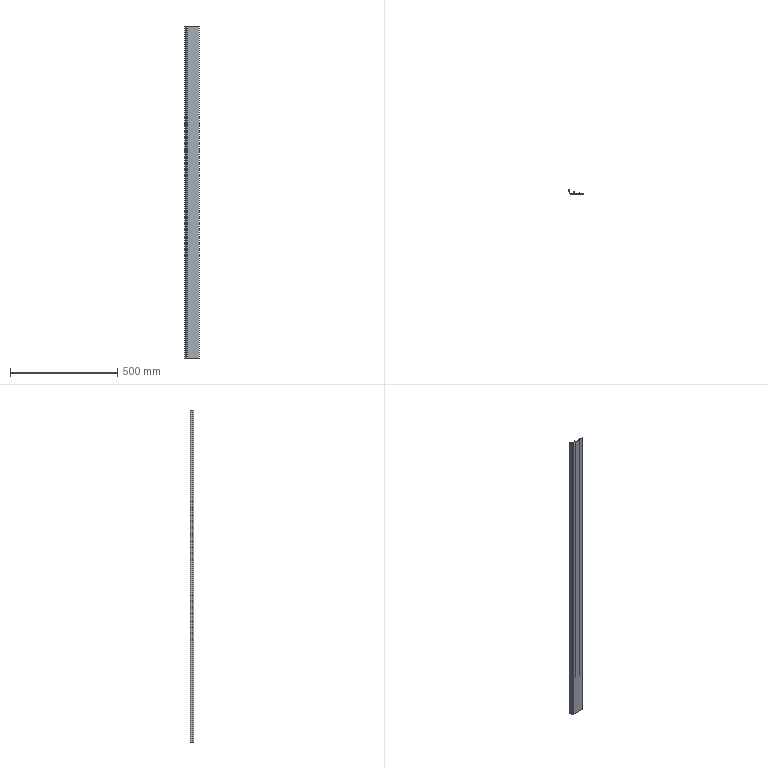Part | STEP file | 51E-01219JG10 | 1 solid | 49 faces | box 67.801 x 18.48 x 1550 mm | volume 173193 mm3 | cylinder 28 | plane 21 | commonest cylinder face diameters 0.4 x11 0.6 x3 1 x3 1.2 x2 1.4 x2 4 x2